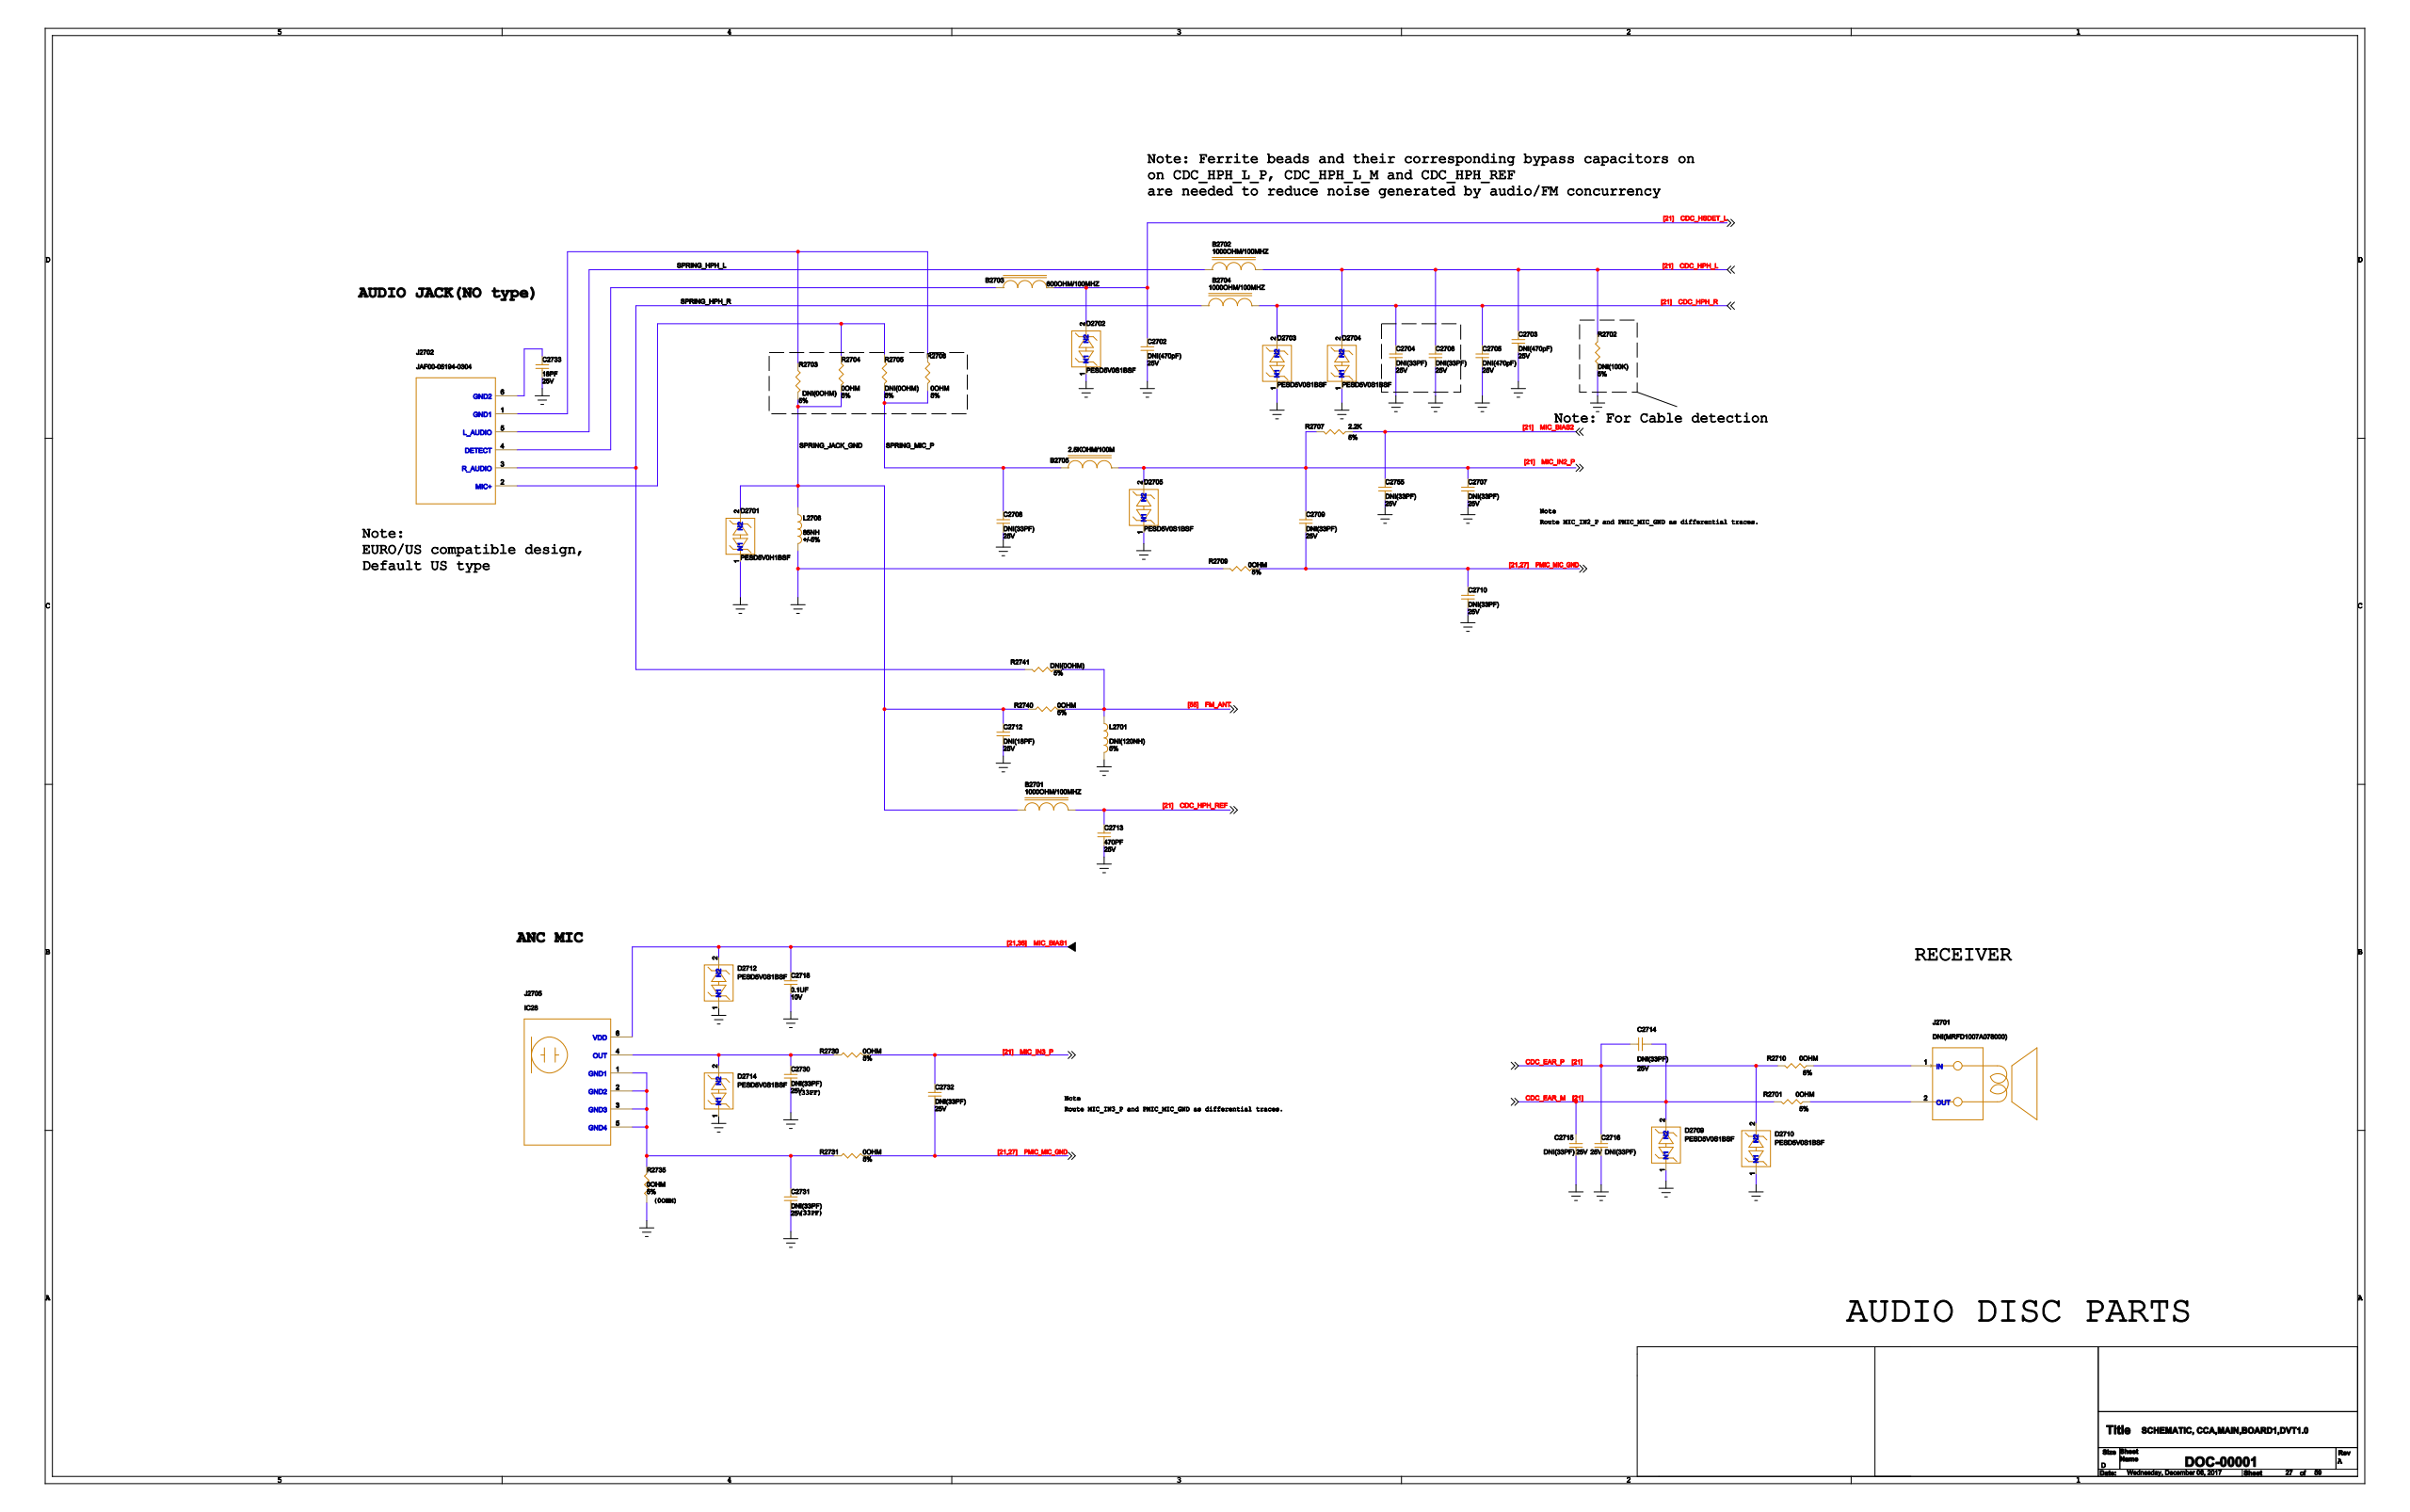Circuit board | KiCad | 1657 parts | 1365 nets | one sheet of the schematic
Parts on this sheet (reference | value | footprint):
B2701
B2702
B2703
B2704
B2705
C2702
C2703
C2704
C2705
C2706
C2707
C2708
C2709
C2710
C2712
C2713
C2714
C2715
C2716
C2718
C2730
C2731
C2732
C2733
C2755
D2701
D2702
D2703
D2704
D2705
D2709
D2710
D2712
D2714
J2701
J2702
J2705
L2701
L2706
R2701
R2702
R2703
R2704
R2705
R2706
R2707
R2709
R2710
R2730
R2731
R2735
R2740
R2741
Nets of these parts (net: part-pin ...):
CDC_EAR_P: C2714-1 C2716-2 D2710-2 R2710-1
N46449254: J2701-1 R2710-2
GND: C2702-2 C2703-2 C2704-2 C2705-2 C2706-2 C2707-2 C2708-2 C2710-2 C2712-2 C2713-2 C2715-1 C2716-1 C2718-2 C2730-2 C2731-2 C2733-2 C2755-2 D2701-1 D2702-1 D2703-1 D2704-1 D2705-1 D2709-1 D2710-1 D2712-1 D2714-1 L2701-2 L2706-2 R2702-2 R2709-1 R2735-2
MIC_BIAS1: C2718-1 D2712-2 J2705-6
SPRING_HPH_R: B2704-1 J2702-3 R2741-1
CDC_HPH_R: B2704-2 C2704-1 C2705-1 D2703-2
CDC_EAR_M: C2714-2 C2715-2 D2709-2 R2701-1
N24387151: C2733-1 J2702-6
SPRING_HPH_L: B2702-1 J2702-5
CDC_HPH_L: B2702-2 C2703-1 C2706-1 D2704-2 R2702-1
N46449252: J2701-2 R2701-2
CDC_HPH_REF: B2701-2 C2713-1
FM_ANT: L2701-1 R2740-2 R2741-2
N22311125: B2703-1 J2702-4
CDC_HSDET_L: B2703-2 C2702-1 D2702-2
PRING_JACK_GND: B2701-1 C2712-1 D2701-2 L2706-1 R2703-1 R2704-1 R2740-1
N22311110: J2702-1 R2703-2 R2706-2
N22311076: J2702-2 R2704-2 R2705-2
SPRING_MIC_P: B2705-1 C2708-1 R2705-1 R2706-1
N21627019: C2730-1 D2714-2 J2705-4 R2730-1
MIC_IN2_P: B2705-2 C2707-1 C2709-1 D2705-2 R2707-1
N21627025: C2731-1 J2705-1 J2705-2 J2705-3 J2705-5 R2731-1 R2735-1
MIC_IN3_P: C2732-1 R2730-2
PMIC_MIC_GND: C2709-2 C2710-1 C2732-2 R2709-2 R2731-2
MIC_BIAS2: C2755-1 R2707-2